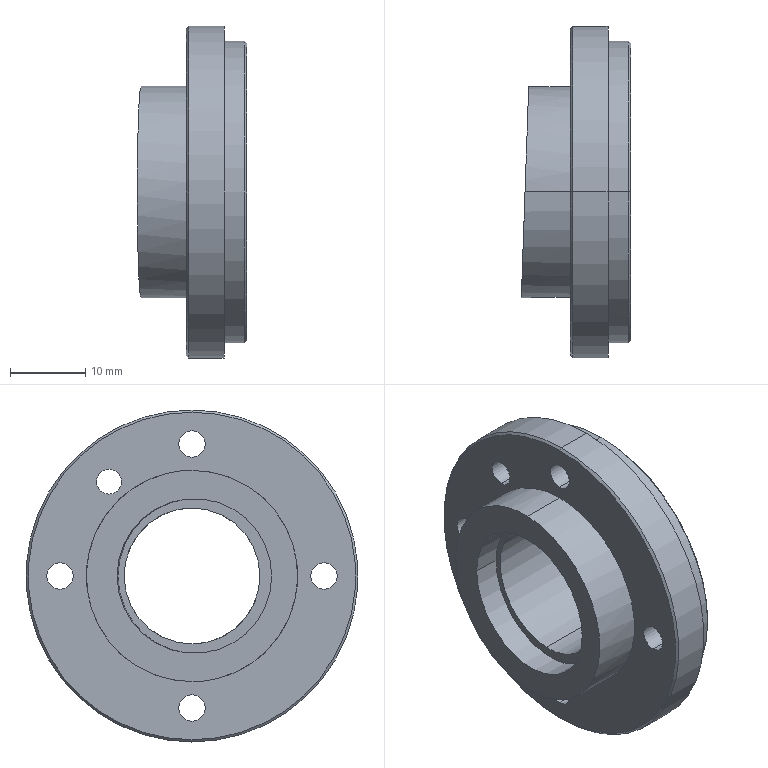Part | SolidWorks | features ICE 5, Chamfer 2, Revolution 1 | 1 solid | 31 faces | box 14.489 x 44 x 44 mm | volume 10850 mm3 | cylinder 20 | cone 6 | plane 5 | commonest cylinder face diameters 3.5 x8 3.3 x2 18 x2 20.5 x2 28 x2 40 x2
STEP:
#1=CARTESIAN_POINT('',(22.7,0.,9.));
#2=VERTEX_POINT('',#1);
#3=CARTESIAN_POINT('',(22.7,0.,-9.));
#4=VERTEX_POINT('',#3);
#5=CARTESIAN_POINT('',(22.7,0.,0.));
#6=DIRECTION('',(1.,0.,0.));
#7=DIRECTION('',(0.,0.,-1.));
#8=AXIS2_PLACEMENT_3D('',#5,#6,#7);
#9=CIRCLE('',#8,9.);
#10=EDGE_CURVE('',#2,#4,#9,.T.);
#11=ORIENTED_EDGE('',*,*,#10,.F.);
#12=CARTESIAN_POINT('',(23.,0.,9.3));
#13=VERTEX_POINT('',#12);
#14=CARTESIAN_POINT('',(22.7,0.,9.));
#15=DIRECTION('',(0.7071,0.,0.7071));
#16=VECTOR('',#15,1000.);
#17=LINE('',#14,#16);
#18=EDGE_CURVE('',#2,#13,#17,.T.);
#19=ORIENTED_EDGE('',*,*,#18,.T.);
#20=CARTESIAN_POINT('',(23.,0.,-9.3));
#21=VERTEX_POINT('',#20);
#22=CARTESIAN_POINT('',(23.,0.,0.));
#23=DIRECTION('',(-1.,0.,0.));
#24=DIRECTION('',(0.,0.,-1.));
#25=AXIS2_PLACEMENT_3D('',#22,#23,#24);
#26=CIRCLE('',#25,9.3);
#27=EDGE_CURVE('',#21,#13,#26,.T.);
#28=ORIENTED_EDGE('',*,*,#27,.F.);
#29=CARTESIAN_POINT('',(22.7,0.,-9.));
#30=DIRECTION('',(0.7071,0.,-0.7071));
#31=VECTOR('',#30,1000.);
#32=LINE('',#29,#31);
#33=EDGE_CURVE('',#4,#21,#32,.T.);
#34=ORIENTED_EDGE('',*,*,#33,.F.);
#35=EDGE_LOOP('',(#11,#19,#28,#34));
#36=FACE_OUTER_BOUND('',#35,.T.);
#37=CARTESIAN_POINT('',(22.7,0.,0.));
#38=DIRECTION('',(1.,0.,0.));
#39=DIRECTION('',(0.,0.,-1.));
#40=AXIS2_PLACEMENT_3D('',#37,#38,#39);
#41=CONICAL_SURFACE('',#40,9.,0.7854);
#42=ADVANCED_FACE('',(#36),#41,.F.);
#43=CARTESIAN_POINT('',(15.,0.,21.7));
#44=VERTEX_POINT('',#43);
#45=CARTESIAN_POINT('',(15.,0.,-21.7));
#46=VERTEX_POINT('',#45);
#47=CARTESIAN_POINT('',(15.,0.,0.));
#48=DIRECTION('',(-1.,0.,0.));
#49=DIRECTION('',(0.,0.,-1.));
#50=AXIS2_PLACEMENT_3D('',#47,#48,#49);
#51=CIRCLE('',#50,21.7);
#52=EDGE_CURVE('',#44,#46,#51,.T.);
#53=ORIENTED_EDGE('',*,*,#52,.F.);
#54=CARTESIAN_POINT('',(15.3,0.,22.));
#55=VERTEX_POINT('',#54);
#56=CARTESIAN_POINT('',(15.,0.,21.7));
#57=DIRECTION('',(0.7071,0.,0.7071));
#58=VECTOR('',#57,1000.);
#59=LINE('',#56,#58);
#60=EDGE_CURVE('',#44,#55,#59,.T.);
#61=ORIENTED_EDGE('',*,*,#60,.T.);
#62=CARTESIAN_POINT('',(15.3,0.,-22.));
#63=VERTEX_POINT('',#62);
#64=CARTESIAN_POINT('',(15.3,0.,0.));
#65=DIRECTION('',(1.,0.,0.));
#66=DIRECTION('',(0.,0.,-1.));
#67=AXIS2_PLACEMENT_3D('',#64,#65,#66);
#68=CIRCLE('',#67,22.);
#69=EDGE_CURVE('',#63,#55,#68,.T.);
#70=ORIENTED_EDGE('',*,*,#69,.F.);
#71=CARTESIAN_POINT('',(15.,0.,-21.7));
#72=DIRECTION('',(0.7071,0.,-0.7071));
#73=VECTOR('',#72,1000.);
#74=LINE('',#71,#73);
#75=EDGE_CURVE('',#46,#63,#74,.T.);
#76=ORIENTED_EDGE('',*,*,#75,.F.);
#77=EDGE_LOOP('',(#53,#61,#70,#76));
#78=FACE_OUTER_BOUND('',#77,.T.);
#79=CARTESIAN_POINT('',(15.,0.,0.));
#80=DIRECTION('',(1.,0.,0.));
#81=DIRECTION('',(0.,0.,-1.));
#82=AXIS2_PLACEMENT_3D('',#79,#80,#81);
#83=CONICAL_SURFACE('',#82,21.7,0.7854);
#84=ADVANCED_FACE('',(#78),#83,.T.);
#85=CARTESIAN_POINT('',(23.,0.,-19.7));
#86=VERTEX_POINT('',#85);
#87=CARTESIAN_POINT('',(23.,0.,19.7));
#88=VERTEX_POINT('',#87);
#89=CARTESIAN_POINT('',(23.,0.,0.));
#90=DIRECTION('',(1.,0.,0.));
#91=DIRECTION('',(0.,0.,-1.));
#92=AXIS2_PLACEMENT_3D('',#89,#90,#91);
#93=CIRCLE('',#92,19.7);
#94=EDGE_CURVE('',#86,#88,#93,.T.);
#95=ORIENTED_EDGE('',*,*,#94,.F.);
#96=CARTESIAN_POINT('',(22.7,0.,-20.));
#97=VERTEX_POINT('',#96);
#98=CARTESIAN_POINT('',(23.,0.,-19.7));
#99=DIRECTION('',(-0.7071,0.,-0.7071));
#100=VECTOR('',#99,1000.);
#101=LINE('',#98,#100);
#102=EDGE_CURVE('',#86,#97,#101,.T.);
#103=ORIENTED_EDGE('',*,*,#102,.T.);
#104=CARTESIAN_POINT('',(22.7,0.,20.));
#105=VERTEX_POINT('',#104);
#106=CARTESIAN_POINT('',(22.7,0.,0.));
#107=DIRECTION('',(-1.,0.,0.));
#108=DIRECTION('',(0.,0.,-1.));
#109=AXIS2_PLACEMENT_3D('',#106,#107,#108);
#110=CIRCLE('',#109,20.);
#111=EDGE_CURVE('',#105,#97,#110,.T.);
#112=ORIENTED_EDGE('',*,*,#111,.F.);
#113=CARTESIAN_POINT('',(23.,0.,19.7));
#114=DIRECTION('',(-0.7071,0.,0.7071));
#115=VECTOR('',#114,1000.);
#116=LINE('',#113,#115);
#117=EDGE_CURVE('',#88,#105,#116,.T.);
#118=ORIENTED_EDGE('',*,*,#117,.F.);
#119=EDGE_LOOP('',(#95,#103,#112,#118));
#120=FACE_OUTER_BOUND('',#119,.T.);
#121=CARTESIAN_POINT('',(23.,0.,0.));
#122=DIRECTION('',(-1.,0.,0.));
#123=DIRECTION('',(0.,0.,1.));
#124=AXIS2_PLACEMENT_3D('',#121,#122,#123);
#125=CONICAL_SURFACE('',#124,19.7,0.7854);
#126=ADVANCED_FACE('',(#120),#125,.T.);
#127=CARTESIAN_POINT('',(15.,11.,10.85));
#128=VERTEX_POINT('',#127);
#129=CARTESIAN_POINT('',(15.,11.,14.15));
#130=VERTEX_POINT('',#129);
#131=CARTESIAN_POINT('',(15.,11.,12.5));
#132=DIRECTION('',(-1.,0.,0.));
#133=DIRECTION('',(0.,0.,-1.));
#134=AXIS2_PLACEMENT_3D('',#131,#132,#133);
#135=CIRCLE('',#134,1.65);
#136=EDGE_CURVE('',#128,#130,#135,.T.);
#137=ORIENTED_EDGE('',*,*,#136,.T.);
#138=CARTESIAN_POINT('',(23.,11.,14.15));
#139=VERTEX_POINT('',#138);
#140=CARTESIAN_POINT('',(8.51,11.,14.15));
#141=DIRECTION('',(1.,0.,0.));
#142=VECTOR('',#141,1000.);
#143=LINE('',#140,#142);
#144=EDGE_CURVE('',#130,#139,#143,.T.);
#145=ORIENTED_EDGE('',*,*,#144,.T.);
#146=CARTESIAN_POINT('',(23.,11.,10.85));
#147=VERTEX_POINT('',#146);
#148=CARTESIAN_POINT('',(23.,11.,12.5));
#149=DIRECTION('',(1.,0.,0.));
#150=DIRECTION('',(0.,0.,-1.));
#151=AXIS2_PLACEMENT_3D('',#148,#149,#150);
#152=CIRCLE('',#151,1.65);
#153=EDGE_CURVE('',#139,#147,#152,.T.);
#154=ORIENTED_EDGE('',*,*,#153,.T.);
#155=CARTESIAN_POINT('',(8.51,11.,10.85));
#156=DIRECTION('',(1.,0.,0.));
#157=VECTOR('',#156,1000.);
#158=LINE('',#155,#157);
#159=EDGE_CURVE('',#128,#147,#158,.T.);
#160=ORIENTED_EDGE('',*,*,#159,.F.);
#161=EDGE_LOOP('',(#137,#145,#154,#160));
#162=FACE_OUTER_BOUND('',#161,.T.);
#163=CARTESIAN_POINT('',(8.51,11.,12.5));
#164=DIRECTION('',(1.,0.,0.));
#165=DIRECTION('',(0.,0.,-1.));
#166=AXIS2_PLACEMENT_3D('',#163,#164,#165);
#167=CYLINDRICAL_SURFACE('',#166,1.65);
#168=ADVANCED_FACE('',(#162),#167,.F.);
#169=ORIENTED_EDGE('',*,*,#111,.T.);
#170=CARTESIAN_POINT('',(20.,0.,-20.));
#171=VERTEX_POINT('',#170);
#172=CARTESIAN_POINT('',(23.,0.,-20.));
#173=DIRECTION('',(-1.,0.,0.));
#174=VECTOR('',#173,1000.);
#175=LINE('',#172,#174);
#176=EDGE_CURVE('',#97,#171,#175,.T.);
#177=ORIENTED_EDGE('',*,*,#176,.T.);
#178=CARTESIAN_POINT('',(20.,0.,20.));
#179=VERTEX_POINT('',#178);
#180=CARTESIAN_POINT('',(20.,0.,0.));
#181=DIRECTION('',(1.,0.,0.));
#182=DIRECTION('',(0.,0.,1.));
#183=AXIS2_PLACEMENT_3D('',#180,#181,#182);
#184=CIRCLE('',#183,20.);
#185=EDGE_CURVE('',#171,#179,#184,.T.);
#186=ORIENTED_EDGE('',*,*,#185,.T.);
#187=CARTESIAN_POINT('',(23.,0.,20.));
#188=DIRECTION('',(-1.,0.,0.));
#189=VECTOR('',#188,1000.);
#190=LINE('',#187,#189);
#191=EDGE_CURVE('',#105,#179,#190,.T.);
#192=ORIENTED_EDGE('',*,*,#191,.F.);
#193=EDGE_LOOP('',(#169,#177,#186,#192));
#194=FACE_OUTER_BOUND('',#193,.T.);
#195=CARTESIAN_POINT('',(23.,0.,0.));
#196=DIRECTION('',(-1.,0.,0.));
#197=DIRECTION('',(0.,0.,1.));
#198=AXIS2_PLACEMENT_3D('',#195,#196,#197);
#199=CYLINDRICAL_SURFACE('',#198,20.);
#200=ADVANCED_FACE('',(#194),#199,.T.);
#201=CARTESIAN_POINT('',(23.,0.,-15.75));
#202=VERTEX_POINT('',#201);
#203=CARTESIAN_POINT('',(23.,0.,-19.25));
#204=VERTEX_POINT('',#203);
#205=CARTESIAN_POINT('',(23.,0.,-17.5));
#206=DIRECTION('',(1.,0.,0.));
#207=DIRECTION('',(0.,0.,-1.));
#208=AXIS2_PLACEMENT_3D('',#205,#206,#207);
#209=CIRCLE('',#208,1.75);
#210=EDGE_CURVE('',#202,#204,#209,.T.);
#211=ORIENTED_EDGE('',*,*,#210,.T.);
#212=CARTESIAN_POINT('',(15.,0.,-19.25));
#213=VERTEX_POINT('',#212);
#214=CARTESIAN_POINT('',(24.95,0.,-19.25));
#215=DIRECTION('',(-1.,0.,0.));
#216=VECTOR('',#215,1000.);
#217=LINE('',#214,#216);
#218=EDGE_CURVE('',#204,#213,#217,.T.);
#219=ORIENTED_EDGE('',*,*,#218,.T.);
#220=CARTESIAN_POINT('',(15.,0.,-15.75));
#221=VERTEX_POINT('',#220);
#222=CARTESIAN_POINT('',(15.,0.,-17.5));
#223=DIRECTION('',(-1.,0.,0.));
#224=DIRECTION('',(0.,0.,1.));
#225=AXIS2_PLACEMENT_3D('',#222,#223,#224);
#226=CIRCLE('',#225,1.75);
#227=EDGE_CURVE('',#213,#221,#226,.T.);
#228=ORIENTED_EDGE('',*,*,#227,.T.);
#229=CARTESIAN_POINT('',(24.95,0.,-15.75));
#230=DIRECTION('',(-1.,0.,0.));
#231=VECTOR('',#230,1000.);
#232=LINE('',#229,#231);
#233=EDGE_CURVE('',#202,#221,#232,.T.);
#234=ORIENTED_EDGE('',*,*,#233,.F.);
#235=EDGE_LOOP('',(#211,#219,#228,#234));
#236=FACE_OUTER_BOUND('',#235,.T.);
#237=CARTESIAN_POINT('',(24.95,0.,-17.5));
#238=DIRECTION('',(-1.,0.,0.));
#239=DIRECTION('',(0.,0.,1.));
#240=AXIS2_PLACEMENT_3D('',#237,#238,#239);
#241=CYLINDRICAL_SURFACE('',#240,1.75);
#242=ADVANCED_FACE('',(#236),#241,.F.);
#243=CARTESIAN_POINT('',(23.,17.5,1.75));
#244=VERTEX_POINT('',#243);
#245=CARTESIAN_POINT('',(23.,17.5,-1.75));
#246=VERTEX_POINT('',#245);
#247=CARTESIAN_POINT('',(23.,17.5,0.));
#248=DIRECTION('',(1.,0.,0.));
#249=DIRECTION('',(0.,0.,-1.));
#250=AXIS2_PLACEMENT_3D('',#247,#248,#249);
#251=CIRCLE('',#250,1.75);
#252=EDGE_CURVE('',#244,#246,#251,.T.);
#253=ORIENTED_EDGE('',*,*,#252,.T.);
#254=CARTESIAN_POINT('',(15.,17.5,-1.75));
#255=VERTEX_POINT('',#254);
#256=CARTESIAN_POINT('',(24.95,17.5,-1.75));
#257=DIRECTION('',(-1.,0.,0.));
#258=VECTOR('',#257,1000.);
#259=LINE('',#256,#258);
#260=EDGE_CURVE('',#246,#255,#259,.T.);
#261=ORIENTED_EDGE('',*,*,#260,.T.);
#262=CARTESIAN_POINT('',(15.,17.5,1.75));
#263=VERTEX_POINT('',#262);
#264=CARTESIAN_POINT('',(15.,17.5,0.));
#265=DIRECTION('',(-1.,0.,0.));
#266=DIRECTION('',(0.,0.,1.));
#267=AXIS2_PLACEMENT_3D('',#264,#265,#266);
#268=CIRCLE('',#267,1.75);
#269=EDGE_CURVE('',#255,#263,#268,.T.);
#270=ORIENTED_EDGE('',*,*,#269,.T.);
#271=CARTESIAN_POINT('',(24.95,17.5,1.75));
#272=DIRECTION('',(-1.,0.,0.));
#273=VECTOR('',#272,1000.);
#274=LINE('',#271,#273);
#275=EDGE_CURVE('',#244,#263,#274,.T.);
#276=ORIENTED_EDGE('',*,*,#275,.F.);
#277=EDGE_LOOP('',(#253,#261,#270,#276));
#278=FACE_OUTER_BOUND('',#277,.T.);
#279=CARTESIAN_POINT('',(24.95,17.5,0.));
#280=DIRECTION('',(-1.,0.,0.));
#281=DIRECTION('',(0.,0.,1.));
#282=AXIS2_PLACEMENT_3D('',#279,#280,#281);
#283=CYLINDRICAL_SURFACE('',#282,1.75);
#284=ADVANCED_FACE('',(#278),#283,.F.);
#285=CARTESIAN_POINT('',(23.,0.,19.25));
#286=VERTEX_POINT('',#285);
#287=CARTESIAN_POINT('',(23.,0.,15.75));
#288=VERTEX_POINT('',#287);
#289=CARTESIAN_POINT('',(23.,0.,17.5));
#290=DIRECTION('',(1.,0.,0.));
#291=DIRECTION('',(0.,0.,-1.));
#292=AXIS2_PLACEMENT_3D('',#289,#290,#291);
#293=CIRCLE('',#292,1.75);
#294=EDGE_CURVE('',#286,#288,#293,.T.);
#295=ORIENTED_EDGE('',*,*,#294,.T.);
#296=CARTESIAN_POINT('',(15.,0.,15.75));
#297=VERTEX_POINT('',#296);
#298=CARTESIAN_POINT('',(24.95,0.,15.75));
#299=DIRECTION('',(-1.,0.,0.));
#300=VECTOR('',#299,1000.);
#301=LINE('',#298,#300);
#302=EDGE_CURVE('',#288,#297,#301,.T.);
#303=ORIENTED_EDGE('',*,*,#302,.T.);
#304=CARTESIAN_POINT('',(15.,0.,19.25));
#305=VERTEX_POINT('',#304);
#306=CARTESIAN_POINT('',(15.,0.,17.5));
#307=DIRECTION('',(-1.,0.,0.));
#308=DIRECTION('',(0.,0.,1.));
#309=AXIS2_PLACEMENT_3D('',#306,#307,#308);
#310=CIRCLE('',#309,1.75);
#311=EDGE_CURVE('',#297,#305,#310,.T.);
#312=ORIENTED_EDGE('',*,*,#311,.T.);
#313=CARTESIAN_POINT('',(24.95,0.,19.25));
#314=DIRECTION('',(-1.,0.,0.));
#315=VECTOR('',#314,1000.);
#316=LINE('',#313,#315);
#317=EDGE_CURVE('',#286,#305,#316,.T.);
#318=ORIENTED_EDGE('',*,*,#317,.F.);
#319=EDGE_LOOP('',(#295,#303,#312,#318));
#320=FACE_OUTER_BOUND('',#319,.T.);
#321=CARTESIAN_POINT('',(24.95,0.,17.5));
#322=DIRECTION('',(-1.,0.,0.));
#323=DIRECTION('',(0.,0.,1.));
#324=AXIS2_PLACEMENT_3D('',#321,#322,#323);
#325=CYLINDRICAL_SURFACE('',#324,1.75);
#326=ADVANCED_FACE('',(#320),#325,.F.);
#327=CARTESIAN_POINT('',(23.,-17.5,1.75));
#328=VERTEX_POINT('',#327);
#329=CARTESIAN_POINT('',(23.,-17.5,-1.75));
#330=VERTEX_POINT('',#329);
#331=CARTESIAN_POINT('',(23.,-17.5,0.));
#332=DIRECTION('',(1.,0.,0.));
#333=DIRECTION('',(0.,0.,-1.));
#334=AXIS2_PLACEMENT_3D('',#331,#332,#333);
#335=CIRCLE('',#334,1.75);
#336=EDGE_CURVE('',#328,#330,#335,.T.);
#337=ORIENTED_EDGE('',*,*,#336,.T.);
#338=CARTESIAN_POINT('',(15.,-17.5,-1.75));
#339=VERTEX_POINT('',#338);
#340=CARTESIAN_POINT('',(24.95,-17.5,-1.75));
#341=DIRECTION('',(-1.,0.,0.));
#342=VECTOR('',#341,1000.);
#343=LINE('',#340,#342);
#344=EDGE_CURVE('',#330,#339,#343,.T.);
#345=ORIENTED_EDGE('',*,*,#344,.T.);
#346=CARTESIAN_POINT('',(15.,-17.5,1.75));
#347=VERTEX_POINT('',#346);
#348=CARTESIAN_POINT('',(15.,-17.5,0.));
#349=DIRECTION('',(-1.,0.,0.));
#350=DIRECTION('',(0.,0.,1.));
#351=AXIS2_PLACEMENT_3D('',#348,#349,#350);
#352=CIRCLE('',#351,1.75);
#353=EDGE_CURVE('',#339,#347,#352,.T.);
#354=ORIENTED_EDGE('',*,*,#353,.T.);
#355=CARTESIAN_POINT('',(24.95,-17.5,1.75));
#356=DIRECTION('',(-1.,0.,0.));
#357=VECTOR('',#356,1000.);
#358=LINE('',#355,#357);
#359=EDGE_CURVE('',#328,#347,#358,.T.);
#360=ORIENTED_EDGE('',*,*,#359,.F.);
#361=EDGE_LOOP('',(#337,#345,#354,#360));
#362=FACE_OUTER_BOUND('',#361,.T.);
#363=CARTESIAN_POINT('',(24.95,-17.5,0.));
#364=DIRECTION('',(-1.,0.,0.));
#365=DIRECTION('',(0.,0.,1.));
#366=AXIS2_PLACEMENT_3D('',#363,#364,#365);
#367=CYLINDRICAL_SURFACE('',#366,1.75);
#368=ADVANCED_FACE('',(#362),#367,.F.);
#369=CARTESIAN_POINT('',(12.845,9.808,0.));
#370=VERTEX_POINT('',#369);
#371=CARTESIAN_POINT('',(12.129,-10.68,0.));
#372=VERTEX_POINT('',#371);
#373=CARTESIAN_POINT('',(12.487,-0.4361,0.));
#374=DIRECTION('',(-0.9994,0.0349,0.));
#375=DIRECTION('',(-0.0349,-0.9994,0.));
#376=AXIS2_PLACEMENT_3D('',#373,#374,#375);
#377=CIRCLE('',#376,10.25);
#378=EDGE_CURVE('',#370,#372,#377,.T.);
#379=ORIENTED_EDGE('',*,*,#378,.F.);
#380=CARTESIAN_POINT('',(9.347,9.93,0.));
#381=VERTEX_POINT('',#380);
#382=CARTESIAN_POINT('',(12.845,9.808,0.));
#383=DIRECTION('',(-0.9994,0.0349,0.));
#384=VECTOR('',#383,1000.);
#385=LINE('',#382,#384);
#386=EDGE_CURVE('',#370,#381,#385,.T.);
#387=ORIENTED_EDGE('',*,*,#386,.T.);
#388=CARTESIAN_POINT('',(8.631,-10.558,0.));
#389=VERTEX_POINT('',#388);
#390=CARTESIAN_POINT('',(8.989,-0.3139,0.));
#391=DIRECTION('',(-0.9994,0.0349,0.));
#392=DIRECTION('',(-0.0349,-0.9994,0.));
#393=AXIS2_PLACEMENT_3D('',#390,#391,#392);
#394=CIRCLE('',#393,10.25);
#395=EDGE_CURVE('',#381,#389,#394,.T.);
#396=ORIENTED_EDGE('',*,*,#395,.T.);
#397=CARTESIAN_POINT('',(12.129,-10.68,0.));
#398=DIRECTION('',(-0.9994,0.0349,0.));
#399=VECTOR('',#398,1000.);
#400=LINE('',#397,#399);
#401=EDGE_CURVE('',#372,#389,#400,.T.);
#402=ORIENTED_EDGE('',*,*,#401,.F.);
#403=EDGE_LOOP('',(#379,#387,#396,#402));
#404=FACE_OUTER_BOUND('',#403,.T.);
#405=CARTESIAN_POINT('',(12.487,-0.4361,0.));
#406=DIRECTION('',(-0.9994,0.0349,0.));
#407=DIRECTION('',(-0.0349,-0.9994,0.));
#408=AXIS2_PLACEMENT_3D('',#405,#406,#407);
#409=CYLINDRICAL_SURFACE('',#408,10.25);
#410=ADVANCED_FACE('',(#404),#409,.F.);
#411=CARTESIAN_POINT('',(15.,0.,14.));
#412=VERTEX_POINT('',#411);
#413=CARTESIAN_POINT('',(15.,0.,-14.));
#414=VERTEX_POINT('',#413);
#415=CARTESIAN_POINT('',(15.,0.,0.));
#416=DIRECTION('',(-1.,0.,0.));
#417=DIRECTION('',(0.,0.,1.));
#418=AXIS2_PLACEMENT_3D('',#415,#416,#417);
#419=CIRCLE('',#418,14.);
#420=EDGE_CURVE('',#412,#414,#419,.T.);
#421=ORIENTED_EDGE('',*,*,#420,.T.);
#422=CARTESIAN_POINT('',(9.,0.,-14.));
#423=VERTEX_POINT('',#422);
#424=CARTESIAN_POINT('',(0.,0.,-14.));
#425=DIRECTION('',(-1.,0.,0.));
#426=VECTOR('',#425,1000.);
#427=LINE('',#424,#426);
#428=EDGE_CURVE('',#414,#423,#427,.T.);
#429=ORIENTED_EDGE('',*,*,#428,.T.);
#430=CARTESIAN_POINT('',(9.,0.,14.));
#431=VERTEX_POINT('',#430);
#432=CARTESIAN_POINT('',(9.,0.,-14.));
#433=CARTESIAN_POINT('',(9.978,28.,-14.));
#434=CARTESIAN_POINT('',(9.978,28.,14.));
#435=CARTESIAN_POINT('',(9.,0.,14.));
#436=(BOUNDED_CURVE()B_SPLINE_CURVE(3,(#432,#433,#434,#435),.UNSPECIFIED.,.F.,.F.)B_SPLINE_CURVE_WITH_KNOTS((4,4),(1.571,4.712),.UNSPECIFIED.)CURVE()GEOMETRIC_REPRESENTATION_ITEM()RATIONAL_B_SPLINE_CURVE((1.,0.3333,0.3333,1.))REPRESENTATION_ITEM(''));
#437=EDGE_CURVE('',#423,#431,#436,.T.);
#438=ORIENTED_EDGE('',*,*,#437,.T.);
#439=CARTESIAN_POINT('',(0.,0.,14.));
#440=DIRECTION('',(-1.,0.,0.));
#441=VECTOR('',#440,1000.);
#442=LINE('',#439,#441);
#443=EDGE_CURVE('',#412,#431,#442,.T.);
#444=ORIENTED_EDGE('',*,*,#443,.F.);
#445=EDGE_LOOP('',(#421,#429,#438,#444));
#446=FACE_OUTER_BOUND('',#445,.T.);
#447=CARTESIAN_POINT('',(0.,0.,0.));
#448=DIRECTION('',(-1.,0.,0.));
#449=DIRECTION('',(0.,0.,1.));
#450=AXIS2_PLACEMENT_3D('',#447,#448,#449);
#451=CYLINDRICAL_SURFACE('',#450,14.);
#452=ADVANCED_FACE('',(#446),#451,.T.);
#453=CARTESIAN_POINT('',(20.,0.,22.));
#454=VERTEX_POINT('',#453);
#455=CARTESIAN_POINT('',(20.,0.,-22.));
#456=VERTEX_POINT('',#455);
#457=CARTESIAN_POINT('',(20.,0.,0.));
#458=DIRECTION('',(-1.,0.,0.));
#459=DIRECTION('',(0.,0.,1.));
#460=AXIS2_PLACEMENT_3D('',#457,#458,#459);
#461=CIRCLE('',#460,22.);
#462=EDGE_CURVE('',#454,#456,#461,.T.);
#463=ORIENTED_EDGE('',*,*,#462,.T.);
#464=CARTESIAN_POINT('',(0.,0.,-22.));
#465=DIRECTION('',(-1.,0.,0.));
#466=VECTOR('',#465,1000.);
#467=LINE('',#464,#466);
#468=EDGE_CURVE('',#456,#63,#467,.T.);
#469=ORIENTED_EDGE('',*,*,#468,.T.);
#470=ORIENTED_EDGE('',*,*,#69,.T.);
#471=CARTESIAN_POINT('',(0.,0.,22.));
#472=DIRECTION('',(-1.,0.,0.));
#473=VECTOR('',#472,1000.);
#474=LINE('',#471,#473);
#475=EDGE_CURVE('',#454,#55,#474,.T.);
#476=ORIENTED_EDGE('',*,*,#475,.F.);
#477=EDGE_LOOP('',(#463,#469,#470,#476));
#478=FACE_OUTER_BOUND('',#477,.T.);
#479=CARTESIAN_POINT('',(0.,0.,0.));
#480=DIRECTION('',(-1.,0.,0.));
#481=DIRECTION('',(0.,0.,1.));
#482=AXIS2_PLACEMENT_3D('',#479,#480,#481);
#483=CYLINDRICAL_SURFACE('',#482,22.);
#484=ADVANCED_FACE('',(#478),#483,.T.);
#485=ORIENTED_EDGE('',*,*,#10,.T.);
#486=CARTESIAN_POINT('',(12.502,0.,-9.));
#487=VERTEX_POINT('',#486);
#488=CARTESIAN_POINT('',(0.,0.,-9.));
#489=DIRECTION('',(-1.,0.,0.));
#490=VECTOR('',#489,1000.);
#491=LINE('',#488,#490);
#492=EDGE_CURVE('',#4,#487,#491,.T.);
#493=ORIENTED_EDGE('',*,*,#492,.T.);
#494=CARTESIAN_POINT('',(12.502,0.,9.));
#495=VERTEX_POINT('',#494);
#496=CARTESIAN_POINT('',(12.502,0.,9.));
#497=CARTESIAN_POINT('',(11.874,-18.,9.));
#498=CARTESIAN_POINT('',(11.874,-18.,-9.));
#499=CARTESIAN_POINT('',(12.502,0.,-9.));
#500=(BOUNDED_CURVE()B_SPLINE_CURVE(3,(#496,#497,#498,#499),.UNSPECIFIED.,.F.,.F.)B_SPLINE_CURVE_WITH_KNOTS((4,4),(4.712,7.854),.UNSPECIFIED.)CURVE()GEOMETRIC_REPRESENTATION_ITEM()RATIONAL_B_SPLINE_CURVE((1.,0.3333,0.3333,1.))REPRESENTATION_ITEM(''));
#501=EDGE_CURVE('',#495,#487,#500,.T.);
#502=ORIENTED_EDGE('',*,*,#501,.F.);
#503=CARTESIAN_POINT('',(0.,0.,9.));
#504=DIRECTION('',(-1.,0.,0.));
#505=VECTOR('',#504,1000.);
#506=LINE('',#503,#505);
#507=EDGE_CURVE('',#2,#495,#506,.T.);
#508=ORIENTED_EDGE('',*,*,#507,.F.);
#509=EDGE_LOOP('',(#485,#493,#502,#508));
#510=FACE_OUTER_BOUND('',#509,.T.);
#511=CARTESIAN_POINT('',(0.,0.,0.));
#512=DIRECTION('',(-1.,0.,0.));
#513=DIRECTION('',(0.,0.,1.));
#514=AXIS2_PLACEMENT_3D('',#511,#512,#513);
#515=CYLINDRICAL_SURFACE('',#514,9.);
#516=ADVANCED_FACE('',(#510),#515,.F.);
#517=ORIENTED_EDGE('',*,*,#462,.F.);
#518=CARTESIAN_POINT('',(20.,0.,0.));
#519=DIRECTION('',(-1.,0.,0.));
#520=DIRECTION('',(0.,0.,1.));
#521=AXIS2_PLACEMENT_3D('',#518,#519,#520);
#522=CIRCLE('',#521,22.);
#523=EDGE_CURVE('',#456,#454,#522,.T.);
#524=ORIENTED_EDGE('',*,*,#523,.F.);
#525=EDGE_LOOP('',(#517,#524));
#526=FACE_OUTER_BOUND('',#525,.T.);
#527=CARTESIAN_POINT('',(20.,0.,0.));
#528=DIRECTION('',(1.,0.,0.));
#529=DIRECTION('',(0.,0.,1.));
#530=AXIS2_PLACEMENT_3D('',#527,#528,#529);
#531=CIRCLE('',#530,20.);
#532=EDGE_CURVE('',#179,#171,#531,.T.);
#533=ORIENTED_EDGE('',*,*,#532,.F.);
#534=ORIENTED_EDGE('',*,*,#185,.F.);
#535=EDGE_LOOP('',(#533,#534));
#536=FACE_BOUND('',#535,.T.);
#537=CARTESIAN_POINT('',(20.,22.,0.));
#538=DIRECTION('',(-1.,0.,0.));
#539=DIRECTION('',(0.,0.,1.));
#540=AXIS2_PLACEMENT_3D('',#537,#538,#539);
#541=PLANE('',#540);
#542=ADVANCED_FACE('',(#526,#536),#541,.F.);
#543=ORIENTED_EDGE('',*,*,#492,.F.);
#544=CARTESIAN_POINT('',(22.7,0.,0.));
#545=DIRECTION('',(1.,0.,0.));
#546=DIRECTION('',(0.,0.,-1.));
#547=AXIS2_PLACEMENT_3D('',#544,#545,#546);
#548=CIRCLE('',#547,9.);
#549=EDGE_CURVE('',#4,#2,#548,.T.);
#550=ORIENTED_EDGE('',*,*,#549,.T.);
#551=ORIENTED_EDGE('',*,*,#507,.T.);
#552=CARTESIAN_POINT('',(12.502,0.,-9.));
#553=CARTESIAN_POINT('',(13.131,18.,-9.));
#554=CARTESIAN_POINT('',(13.131,18.,9.));
#555=CARTESIAN_POINT('',(12.502,0.,9.));
#556=(BOUNDED_CURVE()B_SPLINE_CURVE(3,(#552,#553,#554,#555),.UNSPECIFIED.,.F.,.F.)B_SPLINE_CURVE_WITH_KNOTS((4,4),(1.571,4.712),.UNSPECIFIED.)CURVE()GEOMETRIC_REPRESENTATION_ITEM()RATIONAL_B_SPLINE_CURVE((1.,0.3333,0.3333,1.))REPRESENTATION_ITEM(''));
#557=EDGE_CURVE('',#487,#495,#556,.T.);
#558=ORIENTED_EDGE('',*,*,#557,.F.);
#559=EDGE_LOOP('',(#543,#550,#551,#558));
#560=FACE_OUTER_BOUND('',#559,.T.);
#561=CARTESIAN_POINT('',(0.,0.,0.));
#562=DIRECTION('',(-1.,0.,0.));
#563=DIRECTION('',(0.,0.,1.));
#564=AXIS2_PLACEMENT_3D('',#561,#562,#563);
#565=CYLINDRICAL_SURFACE('',#564,9.);
#566=ADVANCED_FACE('',(#560),#565,.F.);
#567=CARTESIAN_POINT('',(15.,0.,0.));
#568=DIRECTION('',(-1.,0.,0.));
#569=DIRECTION('',(0.,0.,-1.));
#570=AXIS2_PLACEMENT_3D('',#567,#568,#569);
#571=CIRCLE('',#570,21.7);
#572=EDGE_CURVE('',#46,#44,#571,.T.);
#573=ORIENTED_EDGE('',*,*,#572,.T.);
#574=ORIENTED_EDGE('',*,*,#52,.T.);
#575=EDGE_LOOP('',(#573,#574));
#576=FACE_OUTER_BOUND('',#575,.T.);
#577=ORIENTED_EDGE('',*,*,#136,.F.);
#578=CARTESIAN_POINT('',(15.,11.,12.5));
#579=DIRECTION('',(-1.,0.,0.));
#580=DIRECTION('',(0.,0.,-1.));
#581=AXIS2_PLACEMENT_3D('',#578,#579,#580);
#582=CIRCLE('',#581,1.65);
#583=EDGE_CURVE('',#130,#128,#582,.T.);
#584=ORIENTED_EDGE('',*,*,#583,.F.);
#585=EDGE_LOOP('',(#577,#584));
#586=FACE_BOUND('',#585,.T.);
#587=CARTESIAN_POINT('',(15.,0.,-17.5));
#588=DIRECTION('',(-1.,0.,0.));
#589=DIRECTION('',(0.,0.,1.));
#590=AXIS2_PLACEMENT_3D('',#587,#588,#589);
#591=CIRCLE('',#590,1.75);
#592=EDGE_CURVE('',#221,#213,#591,.T.);
#593=ORIENTED_EDGE('',*,*,#592,.F.);
#594=ORIENTED_EDGE('',*,*,#227,.F.);
#595=EDGE_LOOP('',(#593,#594));
#596=FACE_BOUND('',#595,.T.);
#597=CARTESIAN_POINT('',(15.,17.5,0.));
#598=DIRECTION('',(-1.,0.,0.));
#599=DIRECTION('',(0.,0.,1.));
#600=AXIS2_PLACEMENT_3D('',#597,#598,#599);
#601=CIRCLE('',#600,1.75);
#602=EDGE_CURVE('',#263,#255,#601,.T.);
#603=ORIENTED_EDGE('',*,*,#602,.F.);
#604=ORIENTED_EDGE('',*,*,#269,.F.);
#605=EDGE_LOOP('',(#603,#604));
#606=FACE_BOUND('',#605,.T.);
#607=CARTESIAN_POINT('',(15.,0.,17.5));
#608=DIRECTION('',(-1.,0.,0.));
#609=DIRECTION('',(0.,0.,1.));
#610=AXIS2_PLACEMENT_3D('',#607,#608,#609);
#611=CIRCLE('',#610,1.75);
#612=EDGE_CURVE('',#305,#297,#611,.T.);
#613=ORIENTED_EDGE('',*,*,#612,.F.);
#614=ORIENTED_EDGE('',*,*,#311,.F.);
#615=EDGE_LOOP('',(#613,#614));
#616=FACE_BOUND('',#615,.T.);
#617=CARTESIAN_POINT('',(15.,-17.5,0.));
#618=DIRECTION('',(-1.,0.,0.));
#619=DIRECTION('',(0.,0.,1.));
#620=AXIS2_PLACEMENT_3D('',#617,#618,#619);
#621=CIRCLE('',#620,1.75);
#622=EDGE_CURVE('',#347,#339,#621,.T.);
#623=ORIENTED_EDGE('',*,*,#622,.F.);
#624=ORIENTED_EDGE('',*,*,#353,.F.);
#625=EDGE_LOOP('',(#623,#624));
#626=FACE_BOUND('',#625,.T.);
#627=ORIENTED_EDGE('',*,*,#420,.F.);
#628=CARTESIAN_POINT('',(15.,0.,0.));
#629=DIRECTION('',(-1.,0.,0.));
#630=DIRECTION('',(0.,0.,1.));
#631=AXIS2_PLACEMENT_3D('',#628,#629,#630);
#632=CIRCLE('',#631,14.);
#633=EDGE_CURVE('',#414,#412,#632,.T.);
#634=ORIENTED_EDGE('',*,*,#633,.F.);
#635=EDGE_LOOP('',(#627,#634));
#636=FACE_BOUND('',#635,.T.);
#637=CARTESIAN_POINT('',(15.,14.,0.));
#638=DIRECTION('',(1.,0.,0.));
#639=DIRECTION('',(0.,0.,-1.));
#640=AXIS2_PLACEMENT_3D('',#637,#638,#639);
#641=PLANE('',#640);
#642=ADVANCED_FACE('',(#576,#586,#596,#606,#616,#626,#636),#641,.F.);
#643=ORIENTED_EDGE('',*,*,#468,.F.);
#644=ORIENTED_EDGE('',*,*,#523,.T.);
#645=ORIENTED_EDGE('',*,*,#475,.T.);
#646=CARTESIAN_POINT('',(15.3,0.,0.));
#647=DIRECTION('',(1.,0.,0.));
#648=DIRECTION('',(0.,0.,-1.));
#649=AXIS2_PLACEMENT_3D('',#646,#647,#648);
#650=CIRCLE('',#649,22.);
#651=EDGE_CURVE('',#55,#63,#650,.T.);
#652=ORIENTED_EDGE('',*,*,#651,.T.);
#653=EDGE_LOOP('',(#643,#644,#645,#652));
#654=FACE_OUTER_BOUND('',#653,.T.);
#655=CARTESIAN_POINT('',(0.,0.,0.));
#656=DIRECTION('',(-1.,0.,0.));
#657=DIRECTION('',(0.,0.,1.));
#658=AXIS2_PLACEMENT_3D('',#655,#656,#657);
#659=CYLINDRICAL_SURFACE('',#658,22.);
#660=ADVANCED_FACE('',(#654),#659,.T.);
#661=ORIENTED_EDGE('',*,*,#428,.F.);
#662=ORIENTED_EDGE('',*,*,#633,.T.);
#663=ORIENTED_EDGE('',*,*,#443,.T.);
#664=CARTESIAN_POINT('',(9.,0.,14.));
#665=CARTESIAN_POINT('',(8.022,-28.,14.));
#666=CARTESIAN_POINT('',(8.022,-28.,-14.));
#667=CARTESIAN_POINT('',(9.,0.,-14.));
#668=(BOUNDED_CURVE()B_SPLINE_CURVE(3,(#664,#665,#666,#667),.UNSPECIFIED.,.F.,.F.)B_SPLINE_CURVE_WITH_KNOTS((4,4),(4.712,7.854),.UNSPECIFIED.)CURVE()GEOMETRIC_REPRESENTATION_ITEM()RATIONAL_B_SPLINE_CURVE((1.,0.3333,0.3333,1.))REPRESENTATION_ITEM(''));
#669=EDGE_CURVE('',#431,#423,#668,.T.);
#670=ORIENTED_EDGE('',*,*,#669,.T.);
#671=EDGE_LOOP('',(#661,#662,#663,#670));
#672=FACE_OUTER_BOUND('',#671,.T.);
#673=CARTESIAN_POINT('',(0.,0.,0.));
#674=DIRECTION('',(-1.,0.,0.));
#675=DIRECTION('',(0.,0.,1.));
#676=AXIS2_PLACEMENT_3D('',#673,#674,#675);
#677=CYLINDRICAL_SURFACE('',#676,14.);
#678=ADVANCED_FACE('',(#672),#677,.T.);
#679=CARTESIAN_POINT('',(8.989,-0.3139,0.));
#680=DIRECTION('',(-0.9994,0.0349,0.));
#681=DIRECTION('',(-0.0349,-0.9994,0.));
#682=AXIS2_PLACEMENT_3D('',#679,#680,#681);
#683=CIRCLE('',#682,10.25);
#684=EDGE_CURVE('',#389,#381,#683,.T.);
#685=ORIENTED_EDGE('',*,*,#684,.F.);
#686=ORIENTED_EDGE('',*,*,#395,.F.);
#687=EDGE_LOOP('',(#685,#686));
#688=FACE_BOUND('',#687,.T.);
#689=ORIENTED_EDGE('',*,*,#669,.F.);
#690=ORIENTED_EDGE('',*,*,#437,.F.);
#691=EDGE_LOOP('',(#689,#690));
#692=FACE_OUTER_BOUND('',#691,.T.);
#693=CARTESIAN_POINT('',(9.613,17.563,-15.));
#694=DIRECTION('',(0.9994,-0.0349,0.));
#695=DIRECTION('',(0.0349,0.9994,0.));
#696=AXIS2_PLACEMENT_3D('',#693,#694,#695);
#697=PLANE('',#696);
#698=ADVANCED_FACE('',(#688,#692),#697,.F.);
#699=CARTESIAN_POINT('',(12.487,-0.4361,0.));
#700=DIRECTION('',(-0.9994,0.0349,0.));
#701=DIRECTION('',(-0.0349,-0.9994,0.));
#702=AXIS2_PLACEMENT_3D('',#699,#700,#701);
#703=CIRCLE('',#702,10.25);
#704=EDGE_CURVE('',#372,#370,#703,.T.);
#705=ORIENTED_EDGE('',*,*,#704,.T.);
#706=ORIENTED_EDGE('',*,*,#378,.T.);
#707=EDGE_LOOP('',(#705,#706));
#708=FACE_OUTER_BOUND('',#707,.T.);
#709=ORIENTED_EDGE('',*,*,#501,.T.);
#710=ORIENTED_EDGE('',*,*,#557,.T.);
#711=EDGE_LOOP('',(#709,#710));
#712=FACE_BOUND('',#711,.T.);
#713=CARTESIAN_POINT('',(12.487,-0.4361,0.));
#714=DIRECTION('',(-0.9994,0.0349,0.));
#715=DIRECTION('',(-0.0349,-0.9994,0.));
#716=AXIS2_PLACEMENT_3D('',#713,#714,#715);
#717=PLANE('',#716);
#718=ADVANCED_FACE('',(#708,#712),#717,.T.);
#719=ORIENTED_EDGE('',*,*,#386,.F.);
#720=ORIENTED_EDGE('',*,*,#704,.F.);
#721=ORIENTED_EDGE('',*,*,#401,.T.);
#722=ORIENTED_EDGE('',*,*,#684,.T.);
#723=EDGE_LOOP('',(#719,#720,#721,#722));
#724=FACE_OUTER_BOUND('',#723,.T.);
#725=CARTESIAN_POINT('',(12.487,-0.4361,0.));
#726=DIRECTION('',(-0.9994,0.0349,0.));
#727=DIRECTION('',(-0.0349,-0.9994,0.));
#728=AXIS2_PLACEMENT_3D('',#725,#726,#727);
#729=CYLINDRICAL_SURFACE('',#728,10.25);
#730=ADVANCED_FACE('',(#724),#729,.F.);
#731=ORIENTED_EDGE('',*,*,#344,.F.);
#732=CARTESIAN_POINT('',(23.,-17.5,0.));
#733=DIRECTION('',(1.,0.,0.));
#734=DIRECTION('',(0.,0.,-1.));
#735=AXIS2_PLACEMENT_3D('',#732,#733,#734);
#736=CIRCLE('',#735,1.75);
#737=EDGE_CURVE('',#330,#328,#736,.T.);
#738=ORIENTED_EDGE('',*,*,#737,.T.);
#739=ORIENTED_EDGE('',*,*,#359,.T.);
#740=ORIENTED_EDGE('',*,*,#622,.T.);
#741=EDGE_LOOP('',(#731,#738,#739,#740));
#742=FACE_OUTER_BOUND('',#741,.T.);
#743=CARTESIAN_POINT('',(24.95,-17.5,0.));
#744=DIRECTION('',(-1.,0.,0.));
#745=DIRECTION('',(0.,0.,1.));
#746=AXIS2_PLACEMENT_3D('',#743,#744,#745);
#747=CYLINDRICAL_SURFACE('',#746,1.75);
#748=ADVANCED_FACE('',(#742),#747,.F.);
#749=ORIENTED_EDGE('',*,*,#302,.F.);
#750=CARTESIAN_POINT('',(23.,0.,17.5));
#751=DIRECTION('',(1.,0.,0.));
#752=DIRECTION('',(0.,0.,-1.));
#753=AXIS2_PLACEMENT_3D('',#750,#751,#752);
#754=CIRCLE('',#753,1.75);
#755=EDGE_CURVE('',#288,#286,#754,.T.);
#756=ORIENTED_EDGE('',*,*,#755,.T.);
#757=ORIENTED_EDGE('',*,*,#317,.T.);
#758=ORIENTED_EDGE('',*,*,#612,.T.);
#759=EDGE_LOOP('',(#749,#756,#757,#758));
#760=FACE_OUTER_BOUND('',#759,.T.);
#761=CARTESIAN_POINT('',(24.95,0.,17.5));
#762=DIRECTION('',(-1.,0.,0.));
#763=DIRECTION('',(0.,0.,1.));
#764=AXIS2_PLACEMENT_3D('',#761,#762,#763);
#765=CYLINDRICAL_SURFACE('',#764,1.75);
#766=ADVANCED_FACE('',(#760),#765,.F.);
#767=ORIENTED_EDGE('',*,*,#260,.F.);
#768=CARTESIAN_POINT('',(23.,17.5,0.));
#769=DIRECTION('',(1.,0.,0.));
#770=DIRECTION('',(0.,0.,-1.));
#771=AXIS2_PLACEMENT_3D('',#768,#769,#770);
#772=CIRCLE('',#771,1.75);
#773=EDGE_CURVE('',#246,#244,#772,.T.);
#774=ORIENTED_EDGE('',*,*,#773,.T.);
#775=ORIENTED_EDGE('',*,*,#275,.T.);
#776=ORIENTED_EDGE('',*,*,#602,.T.);
#777=EDGE_LOOP('',(#767,#774,#775,#776));
#778=FACE_OUTER_BOUND('',#777,.T.);
#779=CARTESIAN_POINT('',(24.95,17.5,0.));
#780=DIRECTION('',(-1.,0.,0.));
#781=DIRECTION('',(0.,0.,1.));
#782=AXIS2_PLACEMENT_3D('',#779,#780,#781);
#783=CYLINDRICAL_SURFACE('',#782,1.75);
#784=ADVANCED_FACE('',(#778),#783,.F.);
#785=ORIENTED_EDGE('',*,*,#218,.F.);
#786=CARTESIAN_POINT('',(23.,0.,-17.5));
#787=DIRECTION('',(1.,0.,0.));
#788=DIRECTION('',(0.,0.,-1.));
#789=AXIS2_PLACEMENT_3D('',#786,#787,#788);
#790=CIRCLE('',#789,1.75);
#791=EDGE_CURVE('',#204,#202,#790,.T.);
#792=ORIENTED_EDGE('',*,*,#791,.T.);
#793=ORIENTED_EDGE('',*,*,#233,.T.);
#794=ORIENTED_EDGE('',*,*,#592,.T.);
#795=EDGE_LOOP('',(#785,#792,#793,#794));
#796=FACE_OUTER_BOUND('',#795,.T.);
#797=CARTESIAN_POINT('',(24.95,0.,-17.5));
#798=DIRECTION('',(-1.,0.,0.));
#799=DIRECTION('',(0.,0.,1.));
#800=AXIS2_PLACEMENT_3D('',#797,#798,#799);
#801=CYLINDRICAL_SURFACE('',#800,1.75);
#802=ADVANCED_FACE('',(#796),#801,.F.);
#803=ORIENTED_EDGE('',*,*,#27,.T.);
#804=CARTESIAN_POINT('',(23.,0.,0.));
#805=DIRECTION('',(-1.,0.,0.));
#806=DIRECTION('',(0.,0.,-1.));
#807=AXIS2_PLACEMENT_3D('',#804,#805,#806);
#808=CIRCLE('',#807,9.3);
#809=EDGE_CURVE('',#13,#21,#808,.T.);
#810=ORIENTED_EDGE('',*,*,#809,.T.);
#811=EDGE_LOOP('',(#803,#810));
#812=FACE_BOUND('',#811,.T.);
#813=CARTESIAN_POINT('',(23.,0.,0.));
#814=DIRECTION('',(1.,0.,0.));
#815=DIRECTION('',(0.,0.,-1.));
#816=AXIS2_PLACEMENT_3D('',#813,#814,#815);
#817=CIRCLE('',#816,19.7);
#818=EDGE_CURVE('',#88,#86,#817,.T.);
#819=ORIENTED_EDGE('',*,*,#818,.T.);
#820=ORIENTED_EDGE('',*,*,#94,.T.);
#821=EDGE_LOOP('',(#819,#820));
#822=FACE_OUTER_BOUND('',#821,.T.);
#823=CARTESIAN_POINT('',(23.,11.,12.5));
#824=DIRECTION('',(1.,0.,0.));
#825=DIRECTION('',(0.,0.,-1.));
#826=AXIS2_PLACEMENT_3D('',#823,#824,#825);
#827=CIRCLE('',#826,1.65);
#828=EDGE_CURVE('',#147,#139,#827,.T.);
#829=ORIENTED_EDGE('',*,*,#828,.F.);
#830=ORIENTED_EDGE('',*,*,#153,.F.);
#831=EDGE_LOOP('',(#829,#830));
#832=FACE_BOUND('',#831,.T.);
#833=ORIENTED_EDGE('',*,*,#252,.F.);
#834=ORIENTED_EDGE('',*,*,#773,.F.);
#835=EDGE_LOOP('',(#833,#834));
#836=FACE_BOUND('',#835,.T.);
#837=ORIENTED_EDGE('',*,*,#336,.F.);
#838=ORIENTED_EDGE('',*,*,#737,.F.);
#839=EDGE_LOOP('',(#837,#838));
#840=FACE_BOUND('',#839,.T.);
#841=ORIENTED_EDGE('',*,*,#210,.F.);
#842=ORIENTED_EDGE('',*,*,#791,.F.);
#843=EDGE_LOOP('',(#841,#842));
#844=FACE_BOUND('',#843,.T.);
#845=ORIENTED_EDGE('',*,*,#294,.F.);
#846=ORIENTED_EDGE('',*,*,#755,.F.);
#847=EDGE_LOOP('',(#845,#846));
#848=FACE_BOUND('',#847,.T.);
#849=CARTESIAN_POINT('',(23.,0.,0.));
#850=DIRECTION('',(1.,0.,0.));
#851=DIRECTION('',(0.,0.,-1.));
#852=AXIS2_PLACEMENT_3D('',#849,#850,#851);
#853=PLANE('',#852);
#854=ADVANCED_FACE('',(#812,#822,#832,#836,#840,#844,#848),#853,.T.);
#855=ORIENTED_EDGE('',*,*,#176,.F.);
#856=CARTESIAN_POINT('',(22.7,0.,0.));
#857=DIRECTION('',(-1.,0.,0.));
#858=DIRECTION('',(0.,0.,-1.));
#859=AXIS2_PLACEMENT_3D('',#856,#857,#858);
#860=CIRCLE('',#859,20.);
#861=EDGE_CURVE('',#97,#105,#860,.T.);
#862=ORIENTED_EDGE('',*,*,#861,.T.);
#863=ORIENTED_EDGE('',*,*,#191,.T.);
#864=ORIENTED_EDGE('',*,*,#532,.T.);
#865=EDGE_LOOP('',(#855,#862,#863,#864));
#866=FACE_OUTER_BOUND('',#865,.T.);
#867=CARTESIAN_POINT('',(23.,0.,0.));
#868=DIRECTION('',(-1.,0.,0.));
#869=DIRECTION('',(0.,0.,1.));
#870=AXIS2_PLACEMENT_3D('',#867,#868,#869);
#871=CYLINDRICAL_SURFACE('',#870,20.);
#872=ADVANCED_FACE('',(#866),#871,.T.);
#873=ORIENTED_EDGE('',*,*,#144,.F.);
#874=ORIENTED_EDGE('',*,*,#583,.T.);
#875=ORIENTED_EDGE('',*,*,#159,.T.);
#876=ORIENTED_EDGE('',*,*,#828,.T.);
#877=EDGE_LOOP('',(#873,#874,#875,#876));
#878=FACE_OUTER_BOUND('',#877,.T.);
#879=CARTESIAN_POINT('',(8.51,11.,12.5));
#880=DIRECTION('',(1.,0.,0.));
#881=DIRECTION('',(0.,0.,-1.));
#882=AXIS2_PLACEMENT_3D('',#879,#880,#881);
#883=CYLINDRICAL_SURFACE('',#882,1.65);
#884=ADVANCED_FACE('',(#878),#883,.F.);
#885=ORIENTED_EDGE('',*,*,#102,.F.);
#886=ORIENTED_EDGE('',*,*,#818,.F.);
#887=ORIENTED_EDGE('',*,*,#117,.T.);
#888=ORIENTED_EDGE('',*,*,#861,.F.);
#889=EDGE_LOOP('',(#885,#886,#887,#888));
#890=FACE_OUTER_BOUND('',#889,.T.);
#891=CARTESIAN_POINT('',(23.,0.,0.));
#892=DIRECTION('',(-1.,0.,0.));
#893=DIRECTION('',(0.,0.,1.));
#894=AXIS2_PLACEMENT_3D('',#891,#892,#893);
#895=CONICAL_SURFACE('',#894,19.7,0.7854);
#896=ADVANCED_FACE('',(#890),#895,.T.);
#897=ORIENTED_EDGE('',*,*,#60,.F.);
#898=ORIENTED_EDGE('',*,*,#572,.F.);
#899=ORIENTED_EDGE('',*,*,#75,.T.);
#900=ORIENTED_EDGE('',*,*,#651,.F.);
#901=EDGE_LOOP('',(#897,#898,#899,#900));
#902=FACE_OUTER_BOUND('',#901,.T.);
#903=CARTESIAN_POINT('',(15.,0.,0.));
#904=DIRECTION('',(1.,0.,0.));
#905=DIRECTION('',(0.,0.,-1.));
#906=AXIS2_PLACEMENT_3D('',#903,#904,#905);
#907=CONICAL_SURFACE('',#906,21.7,0.7854);
#908=ADVANCED_FACE('',(#902),#907,.T.);
#909=ORIENTED_EDGE('',*,*,#18,.F.);
#910=ORIENTED_EDGE('',*,*,#549,.F.);
#911=ORIENTED_EDGE('',*,*,#33,.T.);
#912=ORIENTED_EDGE('',*,*,#809,.F.);
#913=EDGE_LOOP('',(#909,#910,#911,#912));
#914=FACE_OUTER_BOUND('',#913,.T.);
#915=CARTESIAN_POINT('',(22.7,0.,0.));
#916=DIRECTION('',(1.,0.,0.));
#917=DIRECTION('',(0.,0.,-1.));
#918=AXIS2_PLACEMENT_3D('',#915,#916,#917);
#919=CONICAL_SURFACE('',#918,9.,0.7854);
#920=ADVANCED_FACE('',(#914),#919,.F.);
#921=CLOSED_SHELL('',(#42,#84,#126,#168,#200,#242,#284,#326,#368,#410,#452,#484,#516,#542,#566,#642,#660,#678,#698,#718,#730,#748,#766,#784,#802,#854,#872,#884,#896,#908,#920));
#922=MANIFOLD_SOLID_BREP('',#921);
#923=CARTESIAN_POINT('',(0.,0.,0.));
#924=DIRECTION('',(0.,0.,1.));
#925=DIRECTION('',(1.,0.,0.));
#926=AXIS2_PLACEMENT_3D('',#923,#924,#925);
#927=(LENGTH_UNIT()NAMED_UNIT(*)SI_UNIT(.MILLI.,.METRE.));
#928=UNCERTAINTY_MEASURE_WITH_UNIT(LENGTH_MEASURE(0.00001),#927,'','');
#929=(NAMED_UNIT(*)PLANE_ANGLE_UNIT()SI_UNIT($,.RADIAN.));
#930=(NAMED_UNIT(*)SI_UNIT($,.STERADIAN.)SOLID_ANGLE_UNIT());
#931=(GEOMETRIC_REPRESENTATION_CONTEXT(3)GLOBAL_UNCERTAINTY_ASSIGNED_CONTEXT((#928))GLOBAL_UNIT_ASSIGNED_CONTEXT((#927,#929,#930))REPRESENTATION_CONTEXT('',''));
#932=ADVANCED_BREP_SHAPE_REPRESENTATION('',(#922,#926),#931);